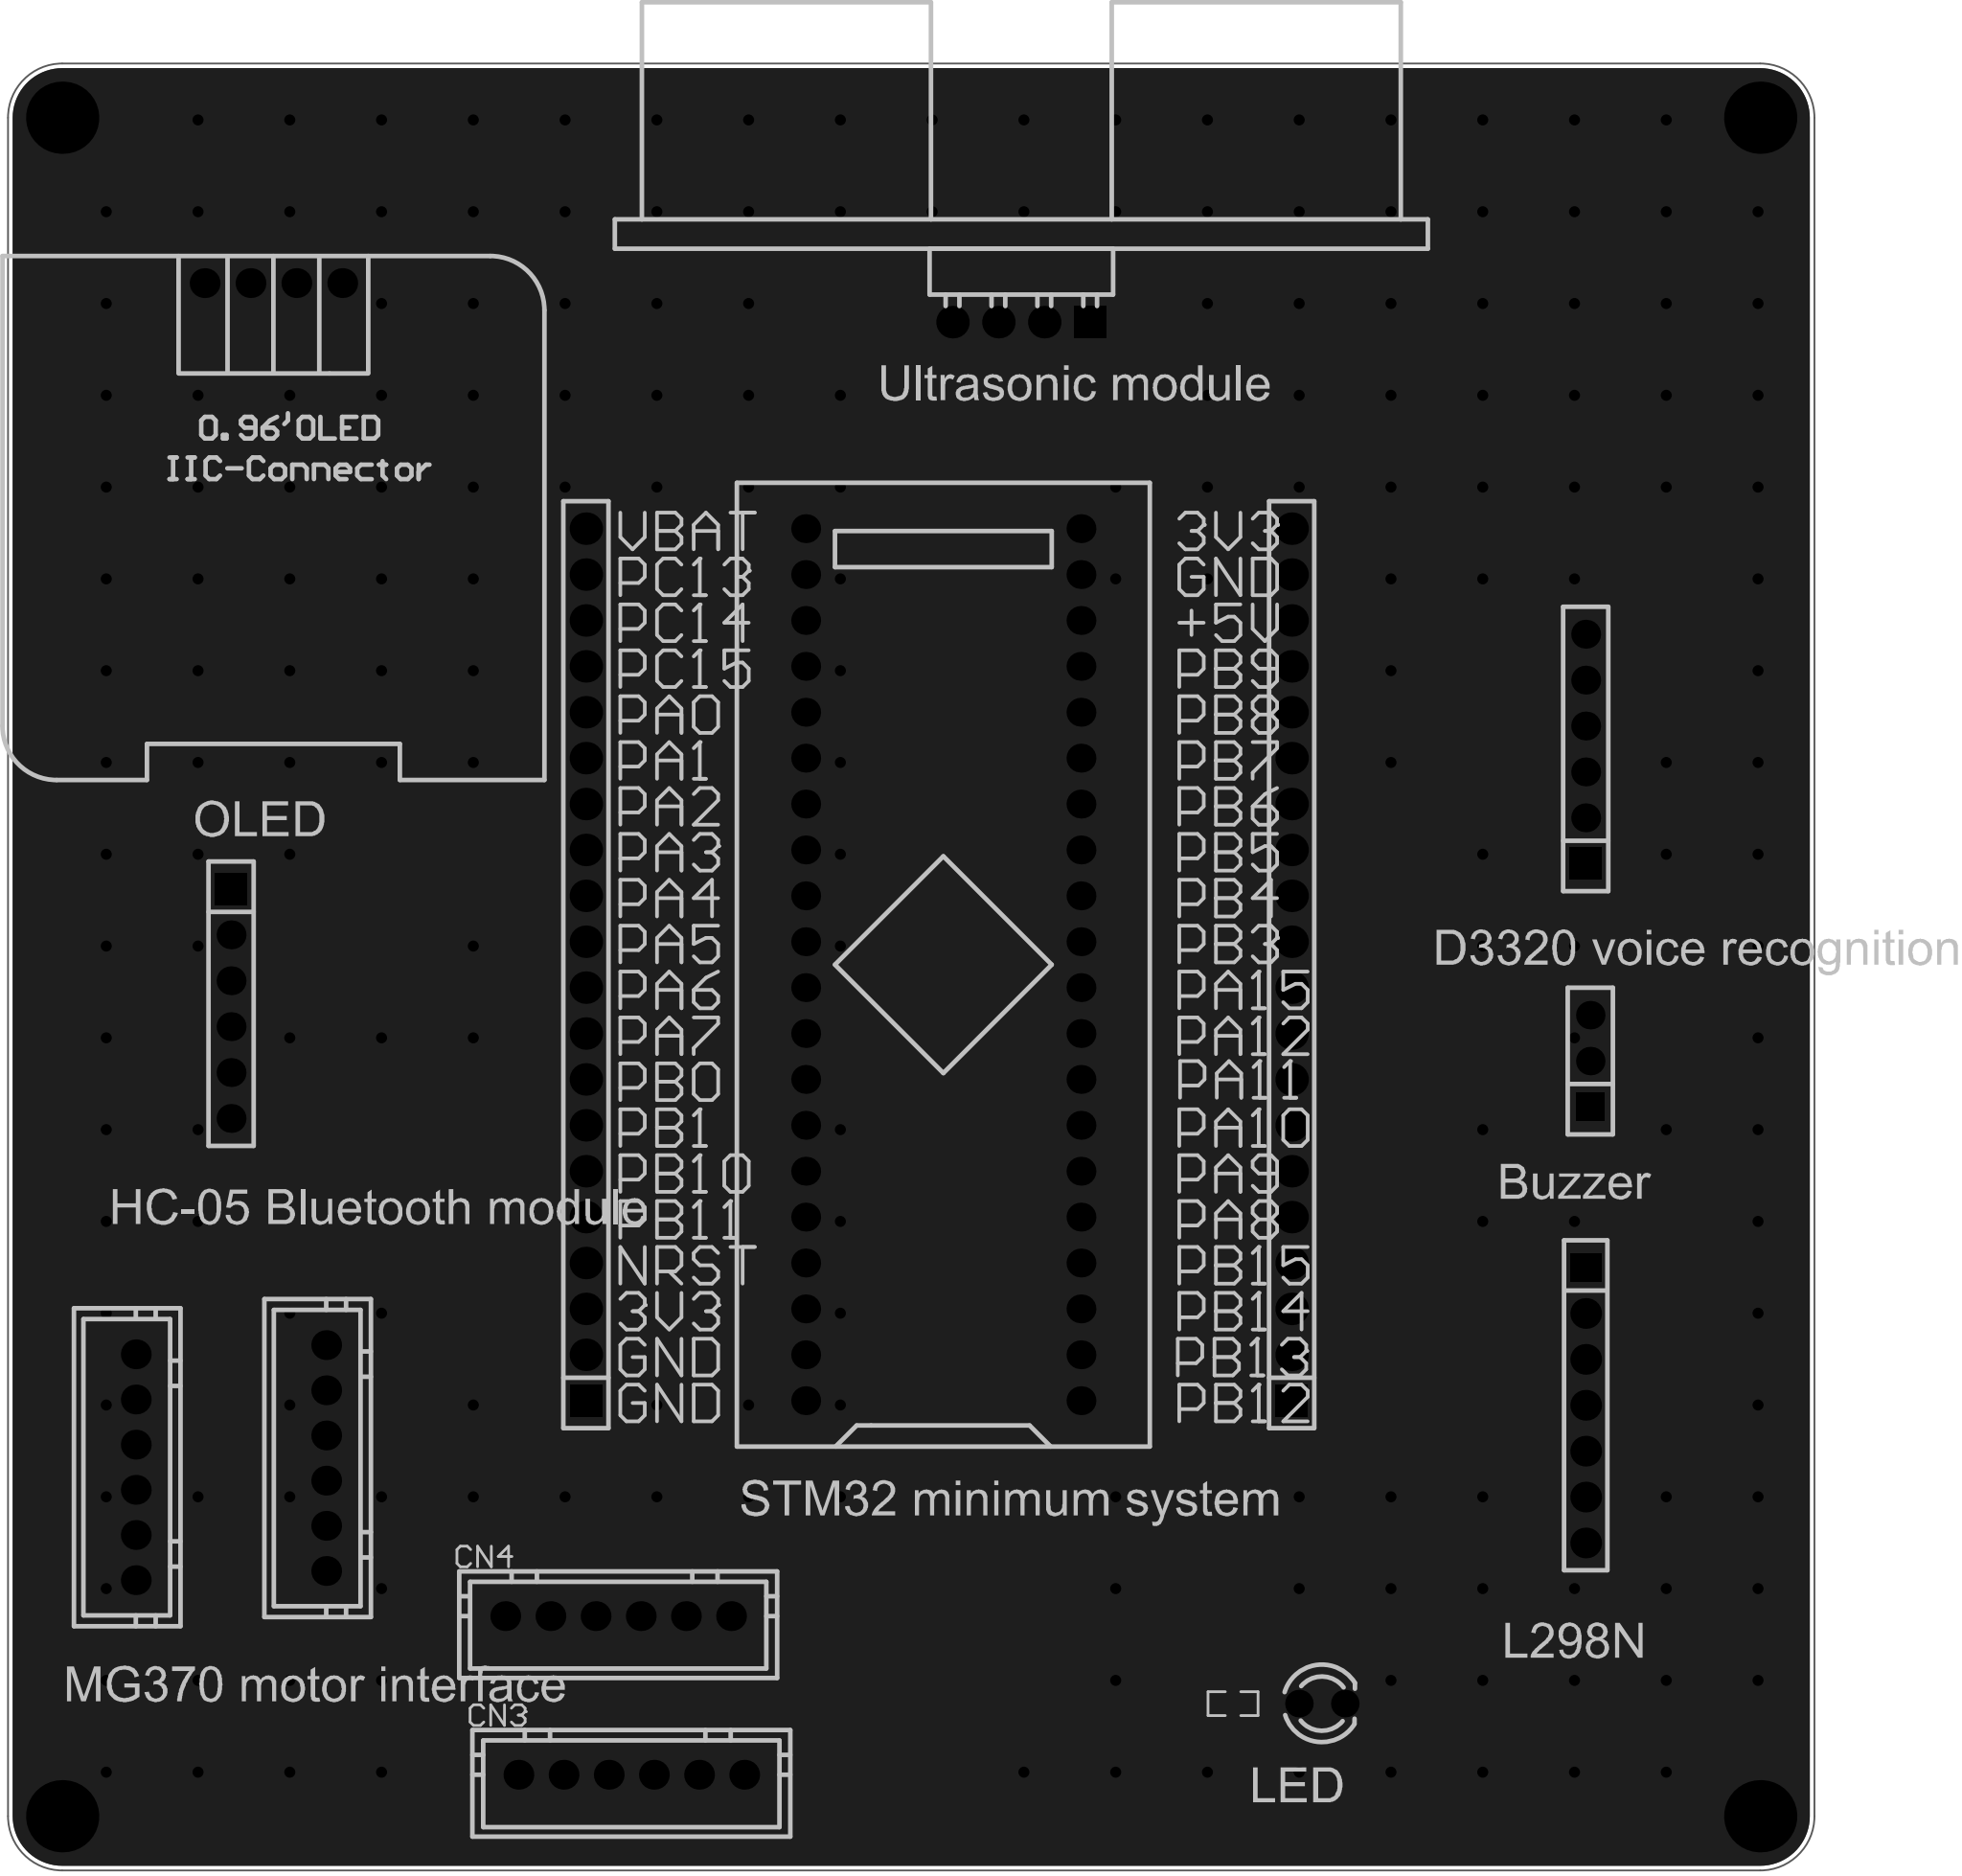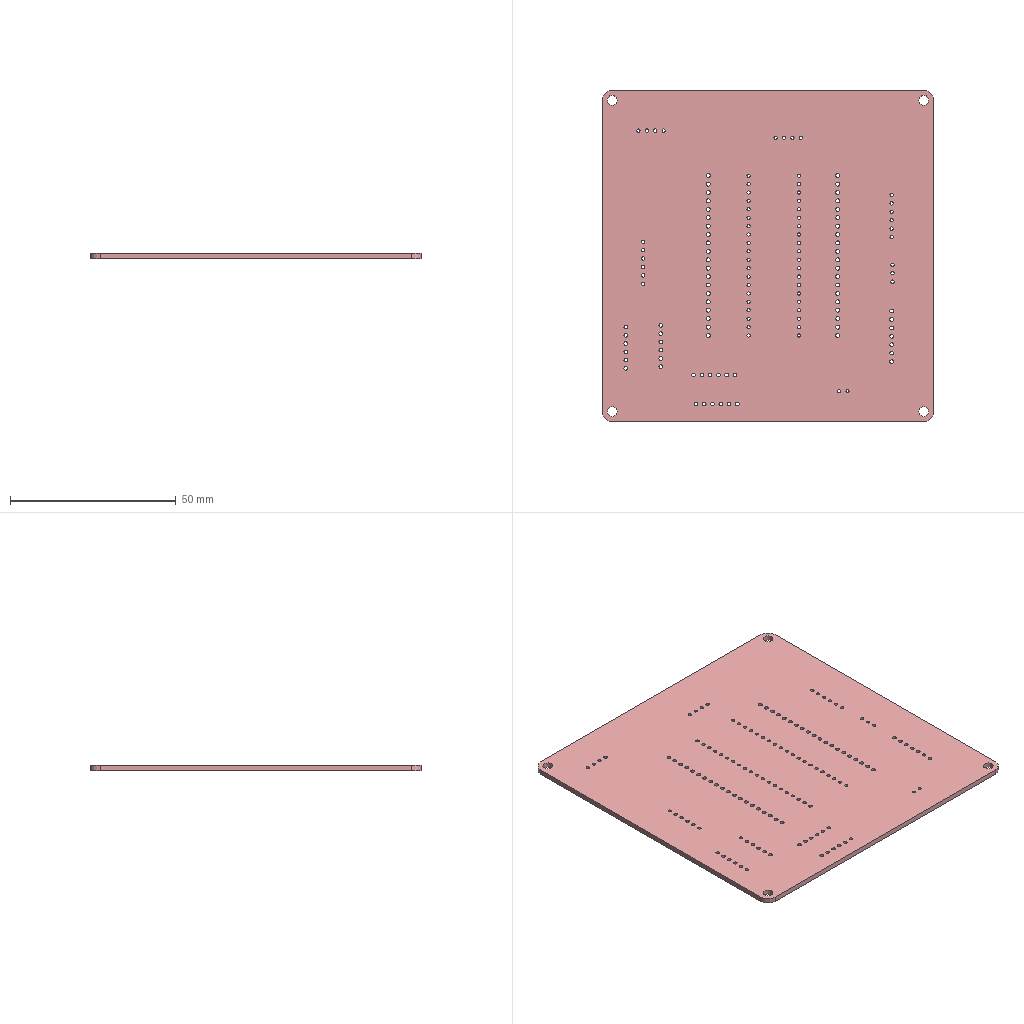Circuit board layout | Altium Designer | box 100 x 100 x 1.6 mm
Layer stack:
# Altium Designer layer stack of  (unit mm; dielectric type: 0 none, 1 core, 2 prepreg, 3 surface material)
index,name,kind,layer,copper_thickness_mm,dielectric_type,dielectric_thickness_mm,dielectric_material,dielectric_constant
0,Top Paste Mask Layer,other,,,,,,
1,Top Silkscreen Layer,other,,,,,,
2,Top Solder Mask Layer,dielectric,,,3,0.01,,3.3
3,Top Layer,copper,Top Layer,0.035,,,,
4,Dielectric1,dielectric,,,3,1.51,FR4,4.5
5,Bottom Layer,copper,Bottom Layer,0.035,,,,
6,Bottom Solder Mask Layer,dielectric,,,3,0.01,,3.3
7,Bottom Silkscreen Layer,other,,,,,,
8,Bottom Paste Mask Layer,other,,,,,,
# drill layer pairs: low layer,high layer
drill_pair,Top Layer,Bottom Layer
Part placement:
Designator,Comment,Layer,Footprint,Center-X(mm),Center-Y(mm),Rotation
U1,STM32F103C8T6-Card,TopLayer,CONN-TH_L53.3-W22.9_STM32F103C8T6-CARD,132.334,129.032,90
H1,,TopLayer,HDR-TH_20P-P2.54-V-F,151.617,129.032,90
H2,,TopLayer,HDR-TH_20P-P2.54-V-F,112.546,129.032,90
H6,,TopLayer,HDR-TH_6P-P2.54-V-F,167.894,140.97,90
H7,,TopLayer,HDR-TH_6P-P2.54-V-F,92.905,126.873,270
CN2,XH2.54*6P_through-hole,TopLayer,CONN-TH_XH2.54-6P,98.171,101.727,270
H8,,TopLayer,HDR-TH_7P-P2.54-V-F,167.894,104.648,270
CN1,XH2.54*6P_through-hole,TopLayer,CONN-TH_XH2.54-6P,87.63,101.219,270
H3,,TopLayer,HDR-TH_3P-P2.54-V-F,168.148,123.698,90
LED1,,TopLayer,LED_TH-3mm,153.289,88.138,0
OLED1,,TopLayer,0.96OLED_4P,95.25,166.751,0
R1,220,TopLayer,R0603,148.371,88.136,180
U2,HC-SR04,TopLayer,TH_HC-SR04V,136.652,164.592,180
CN3,XH2.54*6P_through-hole,TopLayer,CONN-TH_XH2.54-6P,115.062,84.201,0
CN4,XH2.54*6P_through-hole,TopLayer,CONN-TH_XH2.54-6P,114.335,92.98,0
Pad and via stacks:
# Altium Designer via and pad stacks of  (unit mm). Each distinct definition once, with the count of objects using it.
# via: kind,start_layer,end_layer,hole_mm,diameter_mm,mode(0 simple;1 top-mid-bottom;2 full stack),diameter_per_layer,count,example_net
# pad: kind,layer,hole_mm,hole_type(0 round;1 square;2 slot),plating,top_size,top_shape(1 round;2 rect;3 octagon;9 rounded rect),mid_size,bottom_size,mode,footprint,size_per_layer,count,example
pad,Multi-Layer,3,0,plated,4x4,1,4x4,4x4,0,,,4,1
pad,Multi-Layer,1,0,plated,1.6x1.6,1,1.6x1.6,1.6x1.6,0,CONN-TH_L53.3-W22.9_STM32F103C8T6-CARD,,40,U1.1
pad,Multi-Layer,1.2,0,plated,1.8x1.8,2,1.8x1.8,1.8x1.8,0,HDR-TH_20P-P2.54-V-F,,2,H1.1
pad,Multi-Layer,1.2,0,plated,1.8x1.8,1,1.8x1.8,1.8x1.8,0,HDR-TH_20P-P2.54-V-F,,38,H1.2
pad,Multi-Layer,1.02,0,plated,1.6x1.6,1,1.6x1.6,1.6x1.6,0,HDR-TH_6P-P2.54-V-F,,10,H6.6
pad,Multi-Layer,1.02,0,plated,1.8x1.8,2,1.8x1.8,1.8x1.8,0,HDR-TH_6P-P2.54-V-F,,2,H6.1
pad,Multi-Layer,1.1,0,plated,1.65x1.65,1,1.65x1.65,1.65x1.65,0,CONN-TH_XH2.54-6P,,24,CN2.1
pad,Multi-Layer,1.1,0,plated,1.7x1.7,1,1.7x1.7,1.7x1.7,0,HDR-TH_7P-P2.54-V-F,,6,H8.7
pad,Multi-Layer,1.1,0,plated,1.575x1.7,2,1.575x1.7,1.575x1.7,0,HDR-TH_7P-P2.54-V-F,,1,H8.1
pad,Multi-Layer,1.02,0,plated,1.575x1.575,1,1.575x1.575,1.575x1.575,0,HDR-TH_3P-P2.54-V-F,,2,H3.3
pad,Multi-Layer,1.02,0,plated,1.575x1.575,2,1.575x1.575,1.575x1.575,0,HDR-TH_3P-P2.54-V-F,,1,H3.1
pad,Multi-Layer,0.9144,0,plated,1.524x1.524,1,1.524x1.524,1.524x1.524,0,LED_TH-3mm,,2,LED1.1
pad,Multi-Layer,1,0,plated,1.65x1.65,1,1.65x1.65,1.65x1.65,0,0.96OLED_4P,,4,OLED1.4
pad,Multi-Layer,1.001,0,plated,1.8x1.8,1,1.8x1.8,1.8x1.8,0,TH_HC-SR04V,,3,U2.4
pad,Multi-Layer,1.001,0,plated,1.8x1.8,2,1.8x1.8,1.8x1.8,0,TH_HC-SR04V,,1,U2.1
pad,Top Layer,0,0,plated,0.8065x0.864,2,0.8065x0.864,0.8065x0.864,0,R0603,,2,R1.2
via,Top Layer,Bottom Layer,0.3048,0.61,0,,202,PA12
Copper pours:
name,layer,net,type(0 solid;1 hatched;2 none)
Bottom Layer-GND,Bottom Layer,GND,0
Top Layer-GND,Top Layer,GND,0